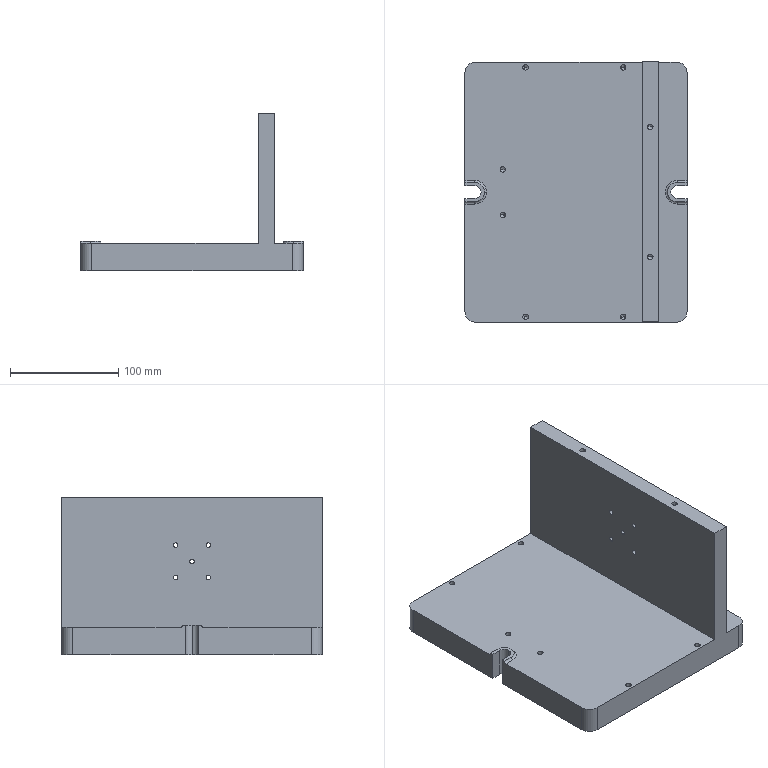Part | SolidWorks | features HoleWzd 4, Fillet 2, ICE 2, Extrusion 1 | 1 solid | 74 faces | box 205 x 240 x 145 mm | volume 1648733 mm3 | cylinder 37 | plane 18 | cone 16 | torus 3 | commonest cylinder face diameters 5 x16 4.2 x10 4 x4 20 x4 12 x3